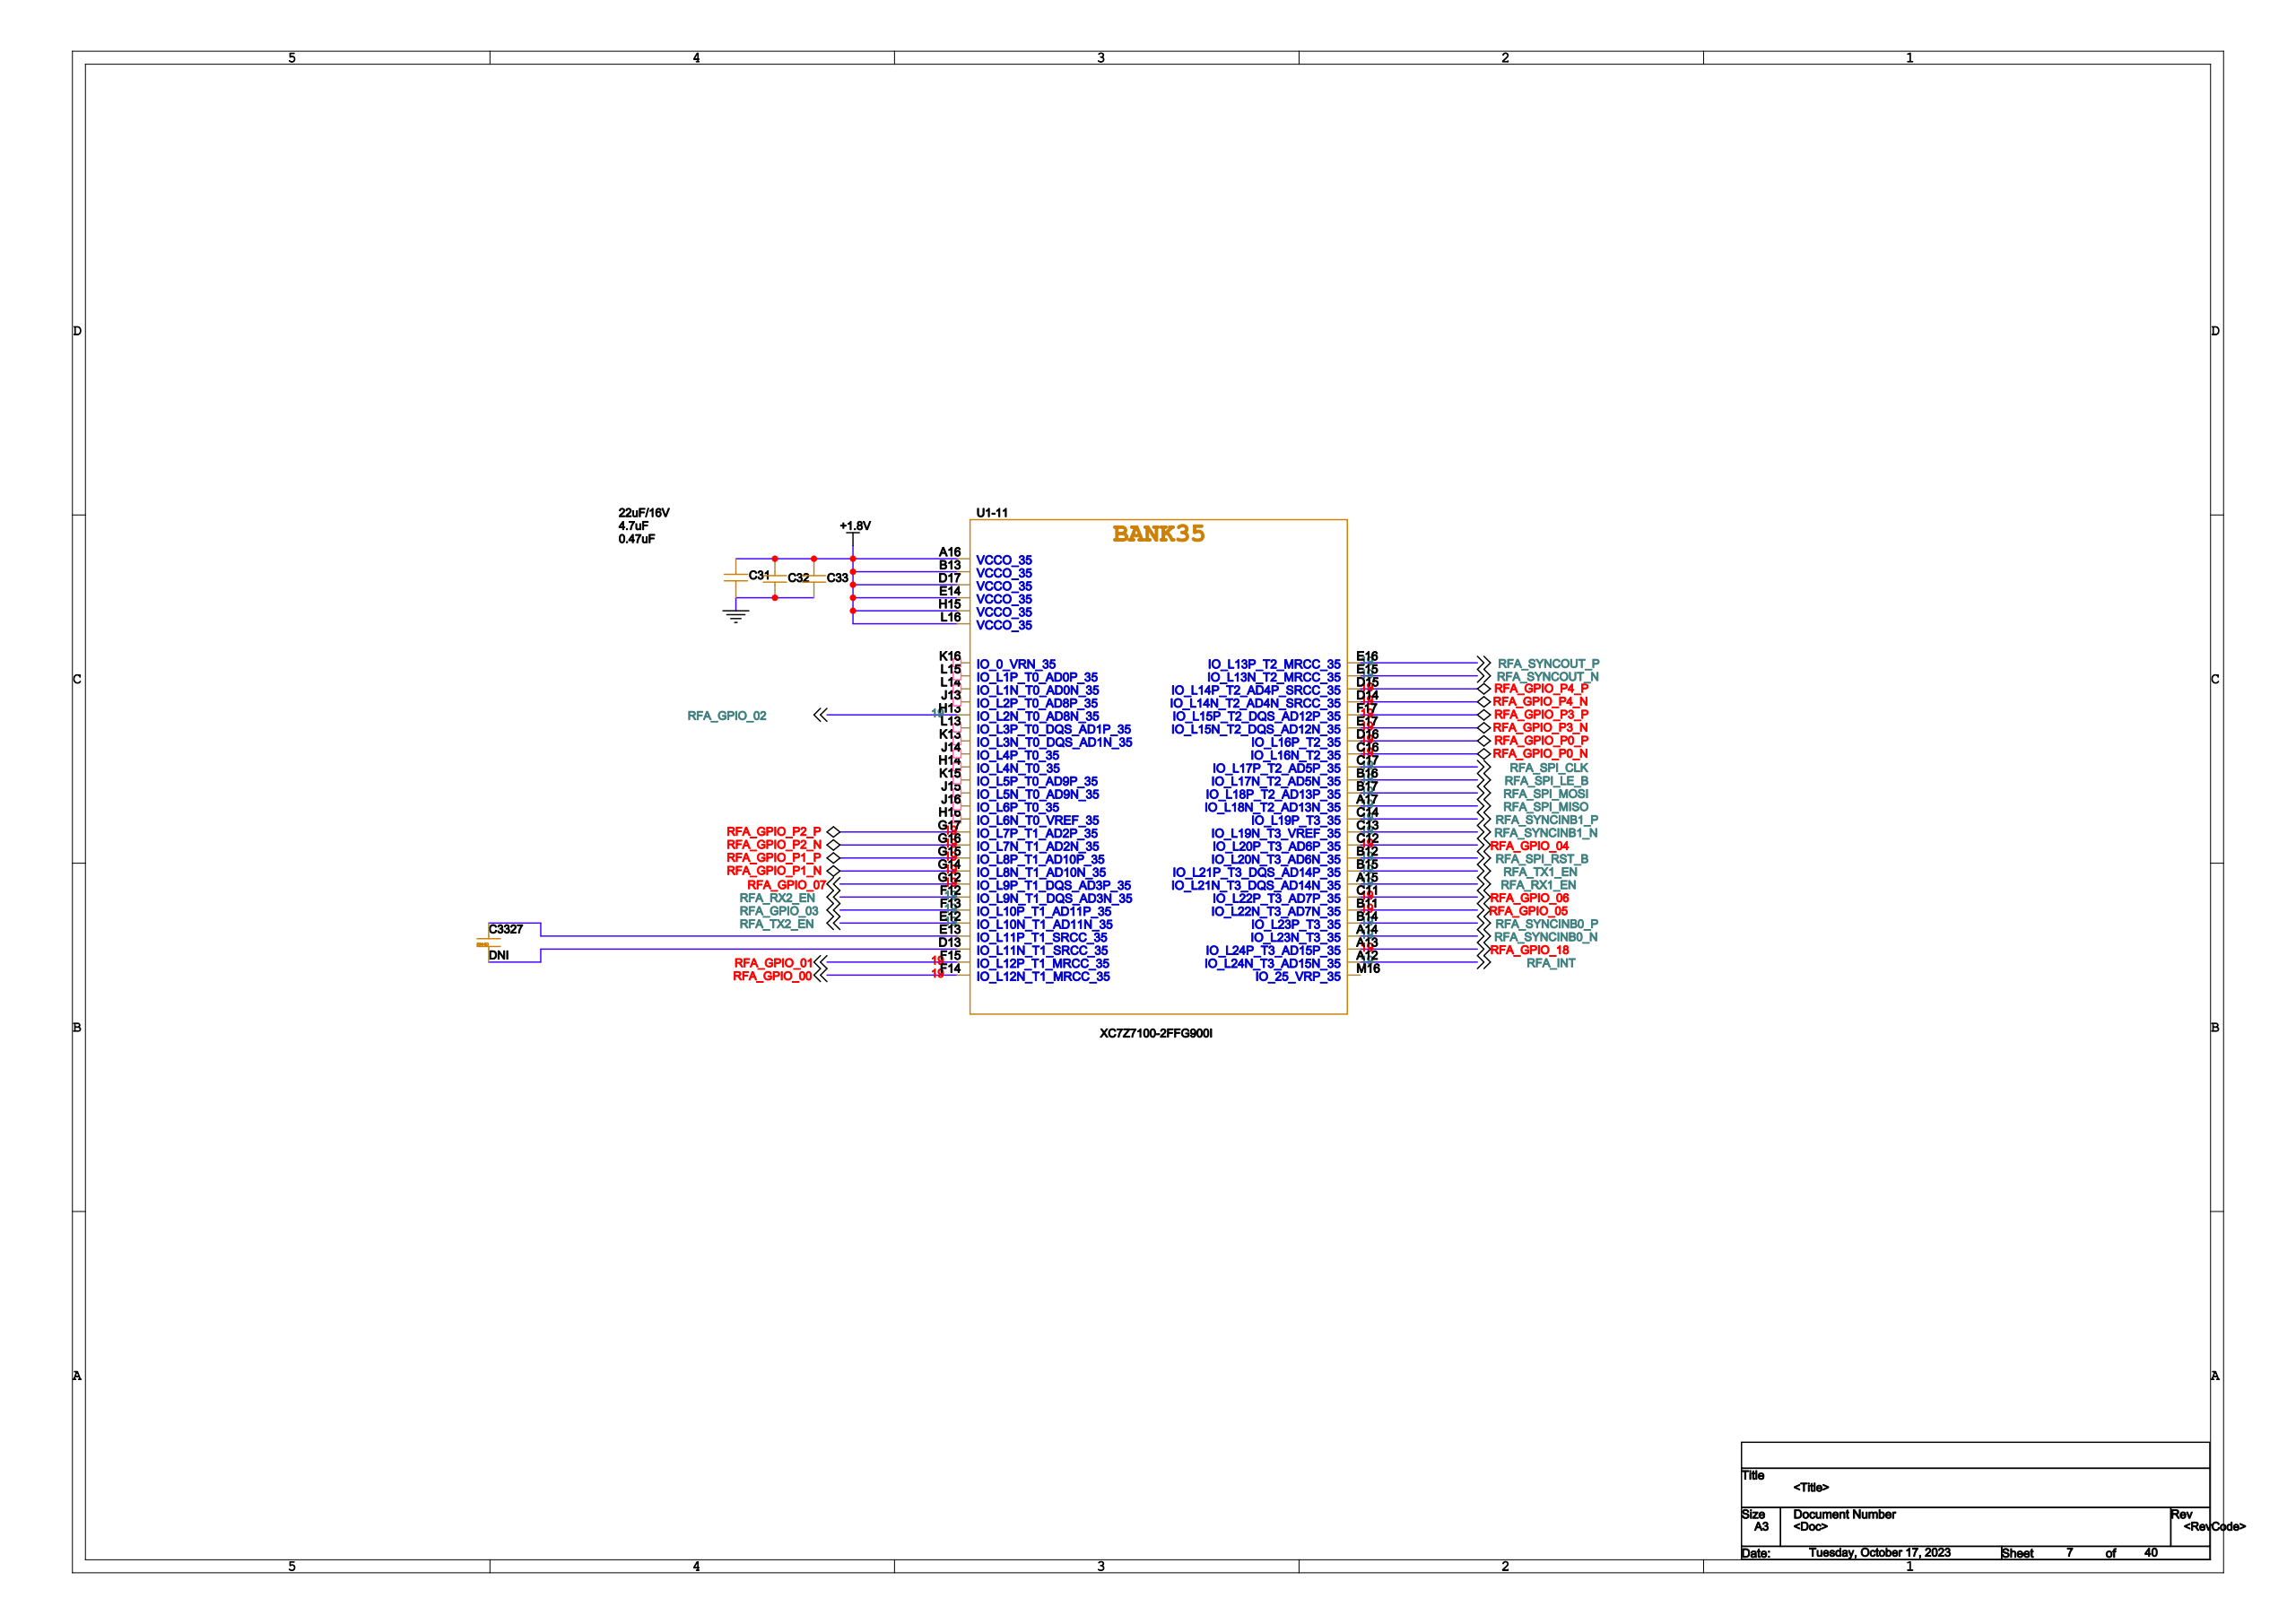Circuit board | Cadence Allegro | 1793 parts | 1223 nets | one sheet of the schematic
Parts on this sheet (reference | value | footprint):
C31 | 22uF/16V | C0603
C32 | 4.7uF | C0402
C33 | 0.47uF | C0402
C3327 | DNI | C0402
Nets of these parts (net: part-pin ...):
GND: C31-2 C32-1 C33-1
+1.8V: C31-1 C32-2 C33-2
N17938343: C3327-1
N17938327: C3327-2